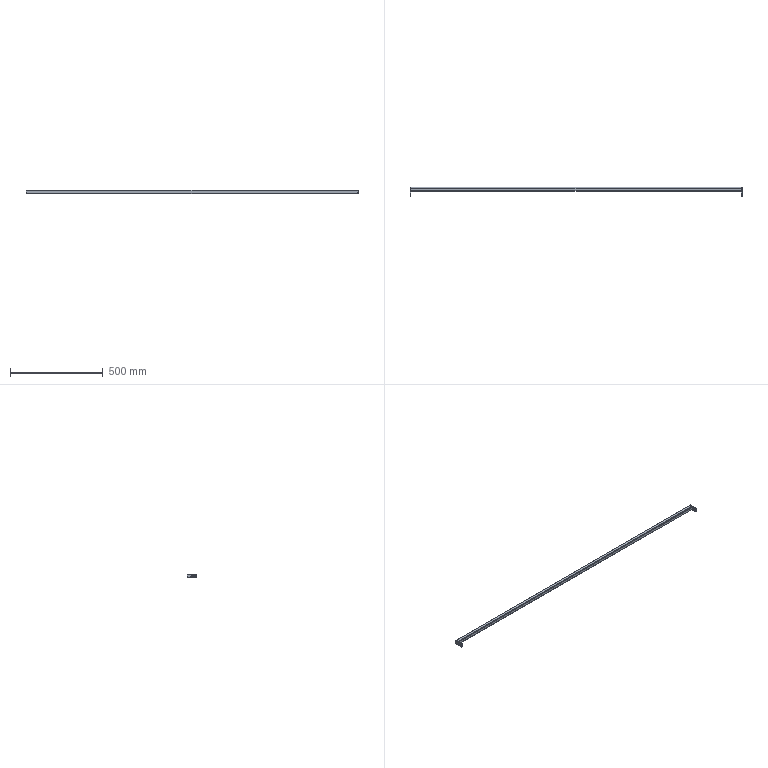Part | SolidWorks | features BaseBody 3 | 3 solids | 46 faces | box 1785 x 50 x 20 mm | volume 245964 mm3 | plane 30 | cylinder 16 | commonest cylinder face diameters 9 x8 4 x4 8 x4
STEP:
#1=CARTESIAN_POINT('',(1780.,-33.,-6.5));
#2=VERTEX_POINT('',#1);
#3=CARTESIAN_POINT('',(1780.,-33.,2.5));
#4=VERTEX_POINT('',#3);
#5=CARTESIAN_POINT('',(1780.,-33.,-2.));
#6=DIRECTION('',(-1.,0.,0.));
#7=DIRECTION('',(0.,0.,1.));
#8=AXIS2_PLACEMENT_3D('',#5,#6,#7);
#9=CIRCLE('',#8,4.5);
#10=EDGE_CURVE('',#2,#4,#9,.T.);
#11=ORIENTED_EDGE('',*,*,#10,.F.);
#12=CARTESIAN_POINT('',(1775.,-33.,-6.5));
#13=VERTEX_POINT('',#12);
#14=CARTESIAN_POINT('',(1775.,-33.,-6.5));
#15=DIRECTION('',(-1.,0.,0.));
#16=VECTOR('',#15,1000.);
#17=LINE('',#14,#16);
#18=EDGE_CURVE('',#2,#13,#17,.T.);
#19=ORIENTED_EDGE('',*,*,#18,.T.);
#20=CARTESIAN_POINT('',(1775.,-33.,2.5));
#21=VERTEX_POINT('',#20);
#22=CARTESIAN_POINT('',(1775.,-33.,-2.));
#23=DIRECTION('',(1.,0.,0.));
#24=DIRECTION('',(0.,0.,1.));
#25=AXIS2_PLACEMENT_3D('',#22,#23,#24);
#26=CIRCLE('',#25,4.5);
#27=EDGE_CURVE('',#21,#13,#26,.T.);
#28=ORIENTED_EDGE('',*,*,#27,.F.);
#29=CARTESIAN_POINT('',(1775.,-33.,2.5));
#30=DIRECTION('',(-1.,0.,0.));
#31=VECTOR('',#30,1000.);
#32=LINE('',#29,#31);
#33=EDGE_CURVE('',#4,#21,#32,.T.);
#34=ORIENTED_EDGE('',*,*,#33,.F.);
#35=EDGE_LOOP('',(#11,#19,#28,#34));
#36=FACE_OUTER_BOUND('',#35,.T.);
#37=CARTESIAN_POINT('',(1775.,-33.,-2.));
#38=DIRECTION('',(-1.,0.,0.));
#39=DIRECTION('',(0.,0.,1.));
#40=AXIS2_PLACEMENT_3D('',#37,#38,#39);
#41=CYLINDRICAL_SURFACE('',#40,4.5);
#42=ADVANCED_FACE('',(#36),#41,.F.);
#43=CARTESIAN_POINT('',(1780.,-18.,-6.5));
#44=VERTEX_POINT('',#43);
#45=CARTESIAN_POINT('',(1780.,-18.,2.5));
#46=VERTEX_POINT('',#45);
#47=CARTESIAN_POINT('',(1780.,-18.,-2.));
#48=DIRECTION('',(-1.,0.,0.));
#49=DIRECTION('',(0.,0.,1.));
#50=AXIS2_PLACEMENT_3D('',#47,#48,#49);
#51=CIRCLE('',#50,4.5);
#52=EDGE_CURVE('',#44,#46,#51,.T.);
#53=ORIENTED_EDGE('',*,*,#52,.F.);
#54=CARTESIAN_POINT('',(1775.,-18.,-6.5));
#55=VERTEX_POINT('',#54);
#56=CARTESIAN_POINT('',(1775.,-18.,-6.5));
#57=DIRECTION('',(-1.,0.,0.));
#58=VECTOR('',#57,1000.);
#59=LINE('',#56,#58);
#60=EDGE_CURVE('',#44,#55,#59,.T.);
#61=ORIENTED_EDGE('',*,*,#60,.T.);
#62=CARTESIAN_POINT('',(1775.,-18.,2.5));
#63=VERTEX_POINT('',#62);
#64=CARTESIAN_POINT('',(1775.,-18.,-2.));
#65=DIRECTION('',(1.,0.,0.));
#66=DIRECTION('',(0.,0.,1.));
#67=AXIS2_PLACEMENT_3D('',#64,#65,#66);
#68=CIRCLE('',#67,4.5);
#69=EDGE_CURVE('',#63,#55,#68,.T.);
#70=ORIENTED_EDGE('',*,*,#69,.F.);
#71=CARTESIAN_POINT('',(1775.,-18.,2.5));
#72=DIRECTION('',(-1.,0.,0.));
#73=VECTOR('',#72,1000.);
#74=LINE('',#71,#73);
#75=EDGE_CURVE('',#46,#63,#74,.T.);
#76=ORIENTED_EDGE('',*,*,#75,.F.);
#77=EDGE_LOOP('',(#53,#61,#70,#76));
#78=FACE_OUTER_BOUND('',#77,.T.);
#79=CARTESIAN_POINT('',(1775.,-18.,-2.));
#80=DIRECTION('',(-1.,0.,0.));
#81=DIRECTION('',(0.,0.,1.));
#82=AXIS2_PLACEMENT_3D('',#79,#80,#81);
#83=CYLINDRICAL_SURFACE('',#82,4.5);
#84=ADVANCED_FACE('',(#78),#83,.F.);
#85=CARTESIAN_POINT('',(1780.,10.,-8.));
#86=VERTEX_POINT('',#85);
#87=CARTESIAN_POINT('',(1780.,10.,8.));
#88=VERTEX_POINT('',#87);
#89=CARTESIAN_POINT('',(1780.,10.,0.));
#90=DIRECTION('',(0.,0.,1.));
#91=VECTOR('',#90,1000.);
#92=LINE('',#89,#91);
#93=EDGE_CURVE('',#86,#88,#92,.T.);
#94=ORIENTED_EDGE('',*,*,#93,.T.);
#95=CARTESIAN_POINT('',(1780.,8.,10.));
#96=VERTEX_POINT('',#95);
#97=CARTESIAN_POINT('',(1780.,10.,8.));
#98=DIRECTION('',(0.,-0.7071,0.7071));
#99=VECTOR('',#98,1000.);
#100=LINE('',#97,#99);
#101=EDGE_CURVE('',#88,#96,#100,.T.);
#102=ORIENTED_EDGE('',*,*,#101,.T.);
#103=CARTESIAN_POINT('',(1780.,-38.,10.));
#104=VERTEX_POINT('',#103);
#105=CARTESIAN_POINT('',(1780.,0.,10.));
#106=DIRECTION('',(0.,-1.,0.));
#107=VECTOR('',#106,1000.);
#108=LINE('',#105,#107);
#109=EDGE_CURVE('',#96,#104,#108,.T.);
#110=ORIENTED_EDGE('',*,*,#109,.T.);
#111=CARTESIAN_POINT('',(1780.,-40.,8.));
#112=VERTEX_POINT('',#111);
#113=CARTESIAN_POINT('',(1780.,-38.,10.));
#114=DIRECTION('',(0.,-0.7071,-0.7071));
#115=VECTOR('',#114,1000.);
#116=LINE('',#113,#115);
#117=EDGE_CURVE('',#104,#112,#116,.T.);
#118=ORIENTED_EDGE('',*,*,#117,.T.);
#119=CARTESIAN_POINT('',(1780.,-40.,-8.));
#120=VERTEX_POINT('',#119);
#121=CARTESIAN_POINT('',(1780.,-40.,0.));
#122=DIRECTION('',(0.,0.,-1.));
#123=VECTOR('',#122,1000.);
#124=LINE('',#121,#123);
#125=EDGE_CURVE('',#112,#120,#124,.T.);
#126=ORIENTED_EDGE('',*,*,#125,.T.);
#127=CARTESIAN_POINT('',(1780.,-38.,-10.));
#128=VERTEX_POINT('',#127);
#129=CARTESIAN_POINT('',(1780.,-40.,-8.));
#130=DIRECTION('',(0.,0.7071,-0.7071));
#131=VECTOR('',#130,1000.);
#132=LINE('',#129,#131);
#133=EDGE_CURVE('',#120,#128,#132,.T.);
#134=ORIENTED_EDGE('',*,*,#133,.T.);
#135=CARTESIAN_POINT('',(1780.,8.,-10.));
#136=VERTEX_POINT('',#135);
#137=CARTESIAN_POINT('',(1780.,0.,-10.));
#138=DIRECTION('',(0.,1.,0.));
#139=VECTOR('',#138,1000.);
#140=LINE('',#137,#139);
#141=EDGE_CURVE('',#128,#136,#140,.T.);
#142=ORIENTED_EDGE('',*,*,#141,.T.);
#143=CARTESIAN_POINT('',(1780.,8.,-10.));
#144=DIRECTION('',(0.,0.7071,0.7071));
#145=VECTOR('',#144,1000.);
#146=LINE('',#143,#145);
#147=EDGE_CURVE('',#136,#86,#146,.T.);
#148=ORIENTED_EDGE('',*,*,#147,.T.);
#149=EDGE_LOOP('',(#94,#102,#110,#118,#126,#134,#142,#148));
#150=FACE_OUTER_BOUND('',#149,.T.);
#151=CARTESIAN_POINT('',(1780.,-33.,-2.));
#152=DIRECTION('',(-1.,0.,0.));
#153=DIRECTION('',(0.,0.,1.));
#154=AXIS2_PLACEMENT_3D('',#151,#152,#153);
#155=CIRCLE('',#154,4.5);
#156=EDGE_CURVE('',#4,#2,#155,.T.);
#157=ORIENTED_EDGE('',*,*,#156,.T.);
#158=ORIENTED_EDGE('',*,*,#10,.T.);
#159=EDGE_LOOP('',(#157,#158));
#160=FACE_BOUND('',#159,.T.);
#161=CARTESIAN_POINT('',(1780.,-18.,-2.));
#162=DIRECTION('',(-1.,0.,0.));
#163=DIRECTION('',(0.,0.,1.));
#164=AXIS2_PLACEMENT_3D('',#161,#162,#163);
#165=CIRCLE('',#164,4.5);
#166=EDGE_CURVE('',#46,#44,#165,.T.);
#167=ORIENTED_EDGE('',*,*,#166,.T.);
#168=ORIENTED_EDGE('',*,*,#52,.T.);
#169=EDGE_LOOP('',(#167,#168));
#170=FACE_BOUND('',#169,.T.);
#171=CARTESIAN_POINT('',(1780.,0.,0.));
#172=DIRECTION('',(1.,0.,0.));
#173=DIRECTION('',(0.,0.,-1.));
#174=AXIS2_PLACEMENT_3D('',#171,#172,#173);
#175=PLANE('',#174);
#176=ADVANCED_FACE('',(#150,#160,#170),#175,.T.);
#177=CARTESIAN_POINT('',(1775.,10.,8.));
#178=VERTEX_POINT('',#177);
#179=CARTESIAN_POINT('',(1780.,10.,8.));
#180=DIRECTION('',(1.,0.,0.));
#181=VECTOR('',#180,1000.);
#182=LINE('',#179,#181);
#183=EDGE_CURVE('',#178,#88,#182,.T.);
#184=ORIENTED_EDGE('',*,*,#183,.F.);
#185=CARTESIAN_POINT('',(1775.,8.,10.));
#186=VERTEX_POINT('',#185);
#187=CARTESIAN_POINT('',(1775.,10.,8.));
#188=DIRECTION('',(0.,0.7071,-0.7071));
#189=VECTOR('',#188,1000.);
#190=LINE('',#187,#189);
#191=EDGE_CURVE('',#186,#178,#190,.T.);
#192=ORIENTED_EDGE('',*,*,#191,.F.);
#193=CARTESIAN_POINT('',(1780.,8.,10.));
#194=DIRECTION('',(-1.,0.,0.));
#195=VECTOR('',#194,1000.);
#196=LINE('',#193,#195);
#197=EDGE_CURVE('',#96,#186,#196,.T.);
#198=ORIENTED_EDGE('',*,*,#197,.F.);
#199=ORIENTED_EDGE('',*,*,#101,.F.);
#200=EDGE_LOOP('',(#184,#192,#198,#199));
#201=FACE_OUTER_BOUND('',#200,.T.);
#202=CARTESIAN_POINT('',(1780.,10.,8.));
#203=DIRECTION('',(0.,-0.7071,-0.7071));
#204=DIRECTION('',(0.,0.7071,-0.7071));
#205=AXIS2_PLACEMENT_3D('',#202,#203,#204);
#206=PLANE('',#205);
#207=ADVANCED_FACE('',(#201),#206,.F.);
#208=CARTESIAN_POINT('',(1775.,10.,-8.));
#209=VERTEX_POINT('',#208);
#210=CARTESIAN_POINT('',(1780.,10.,-8.));
#211=DIRECTION('',(1.,0.,0.));
#212=VECTOR('',#211,1000.);
#213=LINE('',#210,#212);
#214=EDGE_CURVE('',#209,#86,#213,.T.);
#215=ORIENTED_EDGE('',*,*,#214,.F.);
#216=CARTESIAN_POINT('',(1775.,10.,-10.));
#217=DIRECTION('',(0.,0.,-1.));
#218=VECTOR('',#217,1000.);
#219=LINE('',#216,#218);
#220=EDGE_CURVE('',#178,#209,#219,.T.);
#221=ORIENTED_EDGE('',*,*,#220,.F.);
#222=ORIENTED_EDGE('',*,*,#183,.T.);
#223=ORIENTED_EDGE('',*,*,#93,.F.);
#224=EDGE_LOOP('',(#215,#221,#222,#223));
#225=FACE_OUTER_BOUND('',#224,.T.);
#226=CARTESIAN_POINT('',(1780.,10.,-10.));
#227=DIRECTION('',(0.,-1.,0.));
#228=DIRECTION('',(0.,0.,-1.));
#229=AXIS2_PLACEMENT_3D('',#226,#227,#228);
#230=PLANE('',#229);
#231=ADVANCED_FACE('',(#225),#230,.F.);
#232=CARTESIAN_POINT('',(1775.,8.,-10.));
#233=VERTEX_POINT('',#232);
#234=CARTESIAN_POINT('',(1780.,8.,-10.));
#235=DIRECTION('',(1.,0.,0.));
#236=VECTOR('',#235,1000.);
#237=LINE('',#234,#236);
#238=EDGE_CURVE('',#233,#136,#237,.T.);
#239=ORIENTED_EDGE('',*,*,#238,.F.);
#240=CARTESIAN_POINT('',(1775.,8.,-10.));
#241=DIRECTION('',(0.,-0.7071,-0.7071));
#242=VECTOR('',#241,1000.);
#243=LINE('',#240,#242);
#244=EDGE_CURVE('',#209,#233,#243,.T.);
#245=ORIENTED_EDGE('',*,*,#244,.F.);
#246=ORIENTED_EDGE('',*,*,#214,.T.);
#247=ORIENTED_EDGE('',*,*,#147,.F.);
#248=EDGE_LOOP('',(#239,#245,#246,#247));
#249=FACE_OUTER_BOUND('',#248,.T.);
#250=CARTESIAN_POINT('',(1780.,8.,-10.));
#251=DIRECTION('',(0.,-0.7071,0.7071));
#252=DIRECTION('',(0.,-0.7071,-0.7071));
#253=AXIS2_PLACEMENT_3D('',#250,#251,#252);
#254=PLANE('',#253);
#255=ADVANCED_FACE('',(#249),#254,.F.);
#256=CARTESIAN_POINT('',(1775.,-38.,-10.));
#257=VERTEX_POINT('',#256);
#258=CARTESIAN_POINT('',(1780.,-38.,-10.));
#259=DIRECTION('',(1.,0.,0.));
#260=VECTOR('',#259,1000.);
#261=LINE('',#258,#260);
#262=EDGE_CURVE('',#257,#128,#261,.T.);
#263=ORIENTED_EDGE('',*,*,#262,.F.);
#264=CARTESIAN_POINT('',(1775.,10.,-10.));
#265=DIRECTION('',(0.,-1.,0.));
#266=VECTOR('',#265,1000.);
#267=LINE('',#264,#266);
#268=EDGE_CURVE('',#233,#257,#267,.T.);
#269=ORIENTED_EDGE('',*,*,#268,.F.);
#270=ORIENTED_EDGE('',*,*,#238,.T.);
#271=ORIENTED_EDGE('',*,*,#141,.F.);
#272=EDGE_LOOP('',(#263,#269,#270,#271));
#273=FACE_OUTER_BOUND('',#272,.T.);
#274=CARTESIAN_POINT('',(1780.,10.,-10.));
#275=DIRECTION('',(0.,0.,1.));
#276=DIRECTION('',(0.,-1.,0.));
#277=AXIS2_PLACEMENT_3D('',#274,#275,#276);
#278=PLANE('',#277);
#279=ADVANCED_FACE('',(#273),#278,.F.);
#280=CARTESIAN_POINT('',(1775.,-40.,-8.));
#281=VERTEX_POINT('',#280);
#282=CARTESIAN_POINT('',(1780.,-40.,-8.));
#283=DIRECTION('',(1.,0.,0.));
#284=VECTOR('',#283,1000.);
#285=LINE('',#282,#284);
#286=EDGE_CURVE('',#281,#120,#285,.T.);
#287=ORIENTED_EDGE('',*,*,#286,.F.);
#288=CARTESIAN_POINT('',(1775.,-40.,-8.));
#289=DIRECTION('',(0.,-0.7071,0.7071));
#290=VECTOR('',#289,1000.);
#291=LINE('',#288,#290);
#292=EDGE_CURVE('',#257,#281,#291,.T.);
#293=ORIENTED_EDGE('',*,*,#292,.F.);
#294=ORIENTED_EDGE('',*,*,#262,.T.);
#295=ORIENTED_EDGE('',*,*,#133,.F.);
#296=EDGE_LOOP('',(#287,#293,#294,#295));
#297=FACE_OUTER_BOUND('',#296,.T.);
#298=CARTESIAN_POINT('',(1780.,-40.,-8.));
#299=DIRECTION('',(0.,0.7071,0.7071));
#300=DIRECTION('',(0.,-0.7071,0.7071));
#301=AXIS2_PLACEMENT_3D('',#298,#299,#300);
#302=PLANE('',#301);
#303=ADVANCED_FACE('',(#297),#302,.F.);
#304=CARTESIAN_POINT('',(1775.,-40.,8.));
#305=VERTEX_POINT('',#304);
#306=CARTESIAN_POINT('',(1780.,-40.,8.));
#307=DIRECTION('',(1.,0.,0.));
#308=VECTOR('',#307,1000.);
#309=LINE('',#306,#308);
#310=EDGE_CURVE('',#305,#112,#309,.T.);
#311=ORIENTED_EDGE('',*,*,#310,.F.);
#312=CARTESIAN_POINT('',(1775.,-40.,-10.));
#313=DIRECTION('',(0.,0.,1.));
#314=VECTOR('',#313,1000.);
#315=LINE('',#312,#314);
#316=EDGE_CURVE('',#281,#305,#315,.T.);
#317=ORIENTED_EDGE('',*,*,#316,.F.);
#318=ORIENTED_EDGE('',*,*,#286,.T.);
#319=ORIENTED_EDGE('',*,*,#125,.F.);
#320=EDGE_LOOP('',(#311,#317,#318,#319));
#321=FACE_OUTER_BOUND('',#320,.T.);
#322=CARTESIAN_POINT('',(1780.,-40.,-10.));
#323=DIRECTION('',(0.,1.,0.));
#324=DIRECTION('',(0.,0.,1.));
#325=AXIS2_PLACEMENT_3D('',#322,#323,#324);
#326=PLANE('',#325);
#327=ADVANCED_FACE('',(#321),#326,.F.);
#328=CARTESIAN_POINT('',(1775.,-38.,10.));
#329=VERTEX_POINT('',#328);
#330=CARTESIAN_POINT('',(1780.,-38.,10.));
#331=DIRECTION('',(1.,0.,0.));
#332=VECTOR('',#331,1000.);
#333=LINE('',#330,#332);
#334=EDGE_CURVE('',#329,#104,#333,.T.);
#335=ORIENTED_EDGE('',*,*,#334,.F.);
#336=CARTESIAN_POINT('',(1775.,-38.,10.));
#337=DIRECTION('',(0.,0.7071,0.7071));
#338=VECTOR('',#337,1000.);
#339=LINE('',#336,#338);
#340=EDGE_CURVE('',#305,#329,#339,.T.);
#341=ORIENTED_EDGE('',*,*,#340,.F.);
#342=ORIENTED_EDGE('',*,*,#310,.T.);
#343=ORIENTED_EDGE('',*,*,#117,.F.);
#344=EDGE_LOOP('',(#335,#341,#342,#343));
#345=FACE_OUTER_BOUND('',#344,.T.);
#346=CARTESIAN_POINT('',(1780.,-38.,10.));
#347=DIRECTION('',(0.,0.7071,-0.7071));
#348=DIRECTION('',(0.,0.7071,0.7071));
#349=AXIS2_PLACEMENT_3D('',#346,#347,#348);
#350=PLANE('',#349);
#351=ADVANCED_FACE('',(#345),#350,.F.);
#352=ORIENTED_EDGE('',*,*,#334,.T.);
#353=ORIENTED_EDGE('',*,*,#109,.F.);
#354=ORIENTED_EDGE('',*,*,#197,.T.);
#355=CARTESIAN_POINT('',(1775.,10.,10.));
#356=DIRECTION('',(0.,1.,0.));
#357=VECTOR('',#356,1000.);
#358=LINE('',#355,#357);
#359=EDGE_CURVE('',#329,#186,#358,.T.);
#360=ORIENTED_EDGE('',*,*,#359,.F.);
#361=EDGE_LOOP('',(#352,#353,#354,#360));
#362=FACE_OUTER_BOUND('',#361,.T.);
#363=CARTESIAN_POINT('',(1780.,10.,10.));
#364=DIRECTION('',(0.,0.,-1.));
#365=DIRECTION('',(0.,1.,0.));
#366=AXIS2_PLACEMENT_3D('',#363,#364,#365);
#367=PLANE('',#366);
#368=ADVANCED_FACE('',(#362),#367,.F.);
#369=ORIENTED_EDGE('',*,*,#18,.F.);
#370=ORIENTED_EDGE('',*,*,#156,.F.);
#371=ORIENTED_EDGE('',*,*,#33,.T.);
#372=CARTESIAN_POINT('',(1775.,-33.,-2.));
#373=DIRECTION('',(1.,0.,0.));
#374=DIRECTION('',(0.,0.,1.));
#375=AXIS2_PLACEMENT_3D('',#372,#373,#374);
#376=CIRCLE('',#375,4.5);
#377=EDGE_CURVE('',#13,#21,#376,.T.);
#378=ORIENTED_EDGE('',*,*,#377,.F.);
#379=EDGE_LOOP('',(#369,#370,#371,#378));
#380=FACE_OUTER_BOUND('',#379,.T.);
#381=CARTESIAN_POINT('',(1775.,-33.,-2.));
#382=DIRECTION('',(-1.,0.,0.));
#383=DIRECTION('',(0.,0.,1.));
#384=AXIS2_PLACEMENT_3D('',#381,#382,#383);
#385=CYLINDRICAL_SURFACE('',#384,4.5);
#386=ADVANCED_FACE('',(#380),#385,.F.);
#387=ORIENTED_EDGE('',*,*,#60,.F.);
#388=ORIENTED_EDGE('',*,*,#166,.F.);
#389=ORIENTED_EDGE('',*,*,#75,.T.);
#390=CARTESIAN_POINT('',(1775.,-18.,-2.));
#391=DIRECTION('',(1.,0.,0.));
#392=DIRECTION('',(0.,0.,1.));
#393=AXIS2_PLACEMENT_3D('',#390,#391,#392);
#394=CIRCLE('',#393,4.5);
#395=EDGE_CURVE('',#55,#63,#394,.T.);
#396=ORIENTED_EDGE('',*,*,#395,.F.);
#397=EDGE_LOOP('',(#387,#388,#389,#396));
#398=FACE_OUTER_BOUND('',#397,.T.);
#399=CARTESIAN_POINT('',(1775.,-18.,-2.));
#400=DIRECTION('',(-1.,0.,0.));
#401=DIRECTION('',(0.,0.,1.));
#402=AXIS2_PLACEMENT_3D('',#399,#400,#401);
#403=CYLINDRICAL_SURFACE('',#402,4.5);
#404=ADVANCED_FACE('',(#398),#403,.F.);
#405=ORIENTED_EDGE('',*,*,#244,.T.);
#406=ORIENTED_EDGE('',*,*,#268,.T.);
#407=ORIENTED_EDGE('',*,*,#292,.T.);
#408=ORIENTED_EDGE('',*,*,#316,.T.);
#409=ORIENTED_EDGE('',*,*,#340,.T.);
#410=ORIENTED_EDGE('',*,*,#359,.T.);
#411=ORIENTED_EDGE('',*,*,#191,.T.);
#412=ORIENTED_EDGE('',*,*,#220,.T.);
#413=EDGE_LOOP('',(#405,#406,#407,#408,#409,#410,#411,#412));
#414=FACE_OUTER_BOUND('',#413,.T.);
#415=ORIENTED_EDGE('',*,*,#27,.T.);
#416=ORIENTED_EDGE('',*,*,#377,.T.);
#417=EDGE_LOOP('',(#415,#416));
#418=FACE_BOUND('',#417,.T.);
#419=ORIENTED_EDGE('',*,*,#69,.T.);
#420=ORIENTED_EDGE('',*,*,#395,.T.);
#421=EDGE_LOOP('',(#419,#420));
#422=FACE_BOUND('',#421,.T.);
#423=CARTESIAN_POINT('',(1775.,0.,0.));
#424=DIRECTION('',(1.,0.,0.));
#425=DIRECTION('',(0.,0.,-1.));
#426=AXIS2_PLACEMENT_3D('',#423,#424,#425);
#427=PLANE('',#426);
#428=ADVANCED_FACE('',(#414,#418,#422),#427,.F.);
#429=CLOSED_SHELL('',(#42,#84,#176,#207,#231,#255,#279,#303,#327,#351,#368,#386,#404,#428));
#430=MANIFOLD_SOLID_BREP('',#429);
#431=CARTESIAN_POINT('',(-5.,-33.,2.5));
#432=VERTEX_POINT('',#431);
#433=CARTESIAN_POINT('',(-5.,-33.,-6.5));
#434=VERTEX_POINT('',#433);
#435=CARTESIAN_POINT('',(-5.,-33.,-2.));
#436=DIRECTION('',(1.,0.,0.));
#437=DIRECTION('',(0.,0.,-1.));
#438=AXIS2_PLACEMENT_3D('',#435,#436,#437);
#439=CIRCLE('',#438,4.5);
#440=EDGE_CURVE('',#432,#434,#439,.T.);
#441=ORIENTED_EDGE('',*,*,#440,.F.);
#442=CARTESIAN_POINT('',(0.,-33.,2.5));
#443=VERTEX_POINT('',#442);
#444=CARTESIAN_POINT('',(0.,-33.,2.5));
#445=DIRECTION('',(1.,0.,0.));
#446=VECTOR('',#445,1000.);
#447=LINE('',#444,#446);
#448=EDGE_CURVE('',#432,#443,#447,.T.);
#449=ORIENTED_EDGE('',*,*,#448,.T.);
#450=CARTESIAN_POINT('',(0.,-33.,-6.5));
#451=VERTEX_POINT('',#450);
#452=CARTESIAN_POINT('',(0.,-33.,-2.));
#453=DIRECTION('',(1.,0.,0.));
#454=DIRECTION('',(0.,0.,-1.));
#455=AXIS2_PLACEMENT_3D('',#452,#453,#454);
#456=CIRCLE('',#455,4.5);
#457=EDGE_CURVE('',#443,#451,#456,.T.);
#458=ORIENTED_EDGE('',*,*,#457,.T.);
#459=CARTESIAN_POINT('',(0.,-33.,-6.5));
#460=DIRECTION('',(1.,0.,0.));
#461=VECTOR('',#460,1000.);
#462=LINE('',#459,#461);
#463=EDGE_CURVE('',#434,#451,#462,.T.);
#464=ORIENTED_EDGE('',*,*,#463,.F.);
#465=EDGE_LOOP('',(#441,#449,#458,#464));
#466=FACE_OUTER_BOUND('',#465,.T.);
#467=CARTESIAN_POINT('',(0.,-33.,-2.));
#468=DIRECTION('',(1.,0.,0.));
#469=DIRECTION('',(0.,0.,-1.));
#470=AXIS2_PLACEMENT_3D('',#467,#468,#469);
#471=CYLINDRICAL_SURFACE('',#470,4.5);
#472=ADVANCED_FACE('',(#466),#471,.F.);
#473=CARTESIAN_POINT('',(-5.,-18.,2.5));
#474=VERTEX_POINT('',#473);
#475=CARTESIAN_POINT('',(-5.,-18.,-6.5));
#476=VERTEX_POINT('',#475);
#477=CARTESIAN_POINT('',(-5.,-18.,-2.));
#478=DIRECTION('',(1.,0.,0.));
#479=DIRECTION('',(0.,0.,-1.));
#480=AXIS2_PLACEMENT_3D('',#477,#478,#479);
#481=CIRCLE('',#480,4.5);
#482=EDGE_CURVE('',#474,#476,#481,.T.);
#483=ORIENTED_EDGE('',*,*,#482,.F.);
#484=CARTESIAN_POINT('',(0.,-18.,2.5));
#485=VERTEX_POINT('',#484);
#486=CARTESIAN_POINT('',(0.,-18.,2.5));
#487=DIRECTION('',(1.,0.,0.));
#488=VECTOR('',#487,1000.);
#489=LINE('',#486,#488);
#490=EDGE_CURVE('',#474,#485,#489,.T.);
#491=ORIENTED_EDGE('',*,*,#490,.T.);
#492=CARTESIAN_POINT('',(0.,-18.,-6.5));
#493=VERTEX_POINT('',#492);
#494=CARTESIAN_POINT('',(0.,-18.,-2.));
#495=DIRECTION('',(1.,0.,0.));
#496=DIRECTION('',(0.,0.,-1.));
#497=AXIS2_PLACEMENT_3D('',#494,#495,#496);
#498=CIRCLE('',#497,4.5);
#499=EDGE_CURVE('',#485,#493,#498,.T.);
#500=ORIENTED_EDGE('',*,*,#499,.T.);
#501=CARTESIAN_POINT('',(0.,-18.,-6.5));
#502=DIRECTION('',(1.,0.,0.));
#503=VECTOR('',#502,1000.);
#504=LINE('',#501,#503);
#505=EDGE_CURVE('',#476,#493,#504,.T.);
#506=ORIENTED_EDGE('',*,*,#505,.F.);
#507=EDGE_LOOP('',(#483,#491,#500,#506));
#508=FACE_OUTER_BOUND('',#507,.T.);
#509=CARTESIAN_POINT('',(0.,-18.,-2.));
#510=DIRECTION('',(1.,0.,0.));
#511=DIRECTION('',(0.,0.,-1.));
#512=AXIS2_PLACEMENT_3D('',#509,#510,#511);
#513=CYLINDRICAL_SURFACE('',#512,4.5);
#514=ADVANCED_FACE('',(#508),#513,.F.);
#515=CARTESIAN_POINT('',(0.,8.,10.));
#516=VERTEX_POINT('',#515);
#517=CARTESIAN_POINT('',(0.,10.,8.));
#518=VERTEX_POINT('',#517);
#519=CARTESIAN_POINT('',(0.,8.,10.));
#520=DIRECTION('',(0.,0.7071,-0.7071));
#521=VECTOR('',#520,1000.);
#522=LINE('',#519,#521);
#523=EDGE_CURVE('',#516,#518,#522,.T.);
#524=ORIENTED_EDGE('',*,*,#523,.F.);
#525=CARTESIAN_POINT('',(0.,-38.,10.));
#526=VERTEX_POINT('',#525);
#527=CARTESIAN_POINT('',(0.,0.,10.));
#528=DIRECTION('',(0.,1.,0.));
#529=VECTOR('',#528,1000.);
#530=LINE('',#527,#529);
#531=EDGE_CURVE('',#526,#516,#530,.T.);
#532=ORIENTED_EDGE('',*,*,#531,.F.);
#533=CARTESIAN_POINT('',(0.,-40.,8.));
#534=VERTEX_POINT('',#533);
#535=CARTESIAN_POINT('',(0.,-40.,8.));
#536=DIRECTION('',(0.,0.7071,0.7071));
#537=VECTOR('',#536,1000.);
#538=LINE('',#535,#537);
#539=EDGE_CURVE('',#534,#526,#538,.T.);
#540=ORIENTED_EDGE('',*,*,#539,.F.);
#541=CARTESIAN_POINT('',(0.,-40.,-8.));
#542=VERTEX_POINT('',#541);
#543=CARTESIAN_POINT('',(0.,-40.,0.));
#544=DIRECTION('',(0.,0.,1.));
#545=VECTOR('',#544,1000.);
#546=LINE('',#543,#545);
#547=EDGE_CURVE('',#542,#534,#546,.T.);
#548=ORIENTED_EDGE('',*,*,#547,.F.);
#549=CARTESIAN_POINT('',(0.,-38.,-10.));
#550=VERTEX_POINT('',#549);
#551=CARTESIAN_POINT('',(0.,-38.,-10.));
#552=DIRECTION('',(0.,-0.7071,0.7071));
#553=VECTOR('',#552,1000.);
#554=LINE('',#551,#553);
#555=EDGE_CURVE('',#550,#542,#554,.T.);
#556=ORIENTED_EDGE('',*,*,#555,.F.);
#557=CARTESIAN_POINT('',(0.,8.,-10.));
#558=VERTEX_POINT('',#557);
#559=CARTESIAN_POINT('',(0.,0.,-10.));
#560=DIRECTION('',(0.,-1.,0.));
#561=VECTOR('',#560,1000.);
#562=LINE('',#559,#561);
#563=EDGE_CURVE('',#558,#550,#562,.T.);
#564=ORIENTED_EDGE('',*,*,#563,.F.);
#565=CARTESIAN_POINT('',(0.,10.,-8.));
#566=VERTEX_POINT('',#565);
#567=CARTESIAN_POINT('',(0.,10.,-8.));
#568=DIRECTION('',(0.,-0.7071,-0.7071));
#569=VECTOR('',#568,1000.);
#570=LINE('',#567,#569);
#571=EDGE_CURVE('',#566,#558,#570,.T.);
#572=ORIENTED_EDGE('',*,*,#571,.F.);
#573=CARTESIAN_POINT('',(0.,10.,0.));
#574=DIRECTION('',(0.,0.,-1.));
#575=VECTOR('',#574,1000.);
#576=LINE('',#573,#575);
#577=EDGE_CURVE('',#518,#566,#576,.T.);
#578=ORIENTED_EDGE('',*,*,#577,.F.);
#579=EDGE_LOOP('',(#524,#532,#540,#548,#556,#564,#572,#578));
#580=FACE_OUTER_BOUND('',#579,.T.);
#581=CARTESIAN_POINT('',(0.,-33.,-2.));
#582=DIRECTION('',(1.,0.,0.));
#583=DIRECTION('',(0.,0.,-1.));
#584=AXIS2_PLACEMENT_3D('',#581,#582,#583);
#585=CIRCLE('',#584,4.5);
#586=EDGE_CURVE('',#451,#443,#585,.T.);
#587=ORIENTED_EDGE('',*,*,#586,.F.);
#588=ORIENTED_EDGE('',*,*,#457,.F.);
#589=EDGE_LOOP('',(#587,#588));
#590=FACE_BOUND('',#589,.T.);
#591=CARTESIAN_POINT('',(0.,-18.,-2.));
#592=DIRECTION('',(1.,0.,0.));
#593=DIRECTION('',(0.,0.,-1.));
#594=AXIS2_PLACEMENT_3D('',#591,#592,#593);
#595=CIRCLE('',#594,4.5);
#596=EDGE_CURVE('',#493,#485,#595,.T.);
#597=ORIENTED_EDGE('',*,*,#596,.F.);
#598=ORIENTED_EDGE('',*,*,#499,.F.);
#599=EDGE_LOOP('',(#597,#598));
#600=FACE_BOUND('',#599,.T.);
#601=CARTESIAN_POINT('',(0.,0.,0.));
#602=DIRECTION('',(-1.,0.,0.));
#603=DIRECTION('',(0.,0.,1.));
#604=AXIS2_PLACEMENT_3D('',#601,#602,#603);
#605=PLANE('',#604);
#606=ADVANCED_FACE('',(#580,#590,#600),#605,.F.);
#607=CARTESIAN_POINT('',(-5.,10.,8.));
#608=VERTEX_POINT('',#607);
#609=CARTESIAN_POINT('',(-5.,10.,8.));
#610=DIRECTION('',(-1.,0.,0.));
#611=VECTOR('',#610,1000.);
#612=LINE('',#609,#611);
#613=EDGE_CURVE('',#518,#608,#612,.T.);
#614=ORIENTED_EDGE('',*,*,#613,.F.);
#615=ORIENTED_EDGE('',*,*,#577,.T.);
#616=CARTESIAN_POINT('',(-5.,10.,-8.));
#617=VERTEX_POINT('',#616);
#618=CARTESIAN_POINT('',(-5.,10.,-8.));
#619=DIRECTION('',(1.,0.,0.));
#620=VECTOR('',#619,1000.);
#621=LINE('',#618,#620);
#622=EDGE_CURVE('',#617,#566,#621,.T.);
#623=ORIENTED_EDGE('',*,*,#622,.F.);
#624=CARTESIAN_POINT('',(-5.,10.,-10.));
#625=DIRECTION('',(0.,0.,-1.));
#626=VECTOR('',#625,1000.);
#627=LINE('',#624,#626);
#628=EDGE_CURVE('',#608,#617,#627,.T.);
#629=ORIENTED_EDGE('',*,*,#628,.F.);
#630=EDGE_LOOP('',(#614,#615,#623,#629));
#631=FACE_OUTER_BOUND('',#630,.T.);
#632=CARTESIAN_POINT('',(-5.,10.,-10.));
#633=DIRECTION('',(0.,-1.,0.));
#634=DIRECTION('',(0.,0.,-1.));
#635=AXIS2_PLACEMENT_3D('',#632,#633,#634);
#636=PLANE('',#635);
#637=ADVANCED_FACE('',(#631),#636,.F.);
#638=CARTESIAN_POINT('',(-5.,8.,10.));
#639=VERTEX_POINT('',#638);
#640=CARTESIAN_POINT('',(-5.,8.,10.));
#641=DIRECTION('',(-1.,0.,0.));
#642=VECTOR('',#641,1000.);
#643=LINE('',#640,#642);
#644=EDGE_CURVE('',#516,#639,#643,.T.);
#645=ORIENTED_EDGE('',*,*,#644,.F.);
#646=ORIENTED_EDGE('',*,*,#523,.T.);
#647=ORIENTED_EDGE('',*,*,#613,.T.);
#648=CARTESIAN_POINT('',(-5.,10.,8.));
#649=DIRECTION('',(0.,0.7071,-0.7071));
#650=VECTOR('',#649,1000.);
#651=LINE('',#648,#650);
#652=EDGE_CURVE('',#639,#608,#651,.T.);
#653=ORIENTED_EDGE('',*,*,#652,.F.);
#654=EDGE_LOOP('',(#645,#646,#647,#653));
#655=FACE_OUTER_BOUND('',#654,.T.);
#656=CARTESIAN_POINT('',(-5.,10.,8.));
#657=DIRECTION('',(0.,-0.7071,-0.7071));
#658=DIRECTION('',(0.,0.7071,-0.7071));
#659=AXIS2_PLACEMENT_3D('',#656,#657,#658);
#660=PLANE('',#659);
#661=ADVANCED_FACE('',(#655),#660,.F.);
#662=ORIENTED_EDGE('',*,*,#644,.T.);
#663=CARTESIAN_POINT('',(-5.,-38.,10.));
#664=VERTEX_POINT('',#663);
#665=CARTESIAN_POINT('',(-5.,10.,10.));
#666=DIRECTION('',(0.,1.,0.));
#667=VECTOR('',#666,1000.);
#668=LINE('',#665,#667);
#669=EDGE_CURVE('',#664,#639,#668,.T.);
#670=ORIENTED_EDGE('',*,*,#669,.F.);
#671=CARTESIAN_POINT('',(-5.,-38.,10.));
#672=DIRECTION('',(-1.,0.,0.));
#673=VECTOR('',#672,1000.);
#674=LINE('',#671,#673);
#675=EDGE_CURVE('',#526,#664,#674,.T.);
#676=ORIENTED_EDGE('',*,*,#675,.F.);
#677=ORIENTED_EDGE('',*,*,#531,.T.);
#678=EDGE_LOOP('',(#662,#670,#676,#677));
#679=FACE_OUTER_BOUND('',#678,.T.);
#680=CARTESIAN_POINT('',(-5.,10.,10.));
#681=DIRECTION('',(0.,0.,-1.));
#682=DIRECTION('',(0.,1.,0.));
#683=AXIS2_PLACEMENT_3D('',#680,#681,#682);
#684=PLANE('',#683);
#685=ADVANCED_FACE('',(#679),#684,.F.);
#686=CARTESIAN_POINT('',(-5.,-40.,8.));
#687=VERTEX_POINT('',#686);
#688=CARTESIAN_POINT('',(-5.,-40.,8.));
#689=DIRECTION('',(-1.,0.,0.));
#690=VECTOR('',#689,1000.);
#691=LINE('',#688,#690);
#692=EDGE_CURVE('',#534,#687,#691,.T.);
#693=ORIENTED_EDGE('',*,*,#692,.F.);
#694=ORIENTED_EDGE('',*,*,#539,.T.);
#695=ORIENTED_EDGE('',*,*,#675,.T.);
#696=CARTESIAN_POINT('',(-5.,-38.,10.));
#697=DIRECTION('',(0.,0.7071,0.7071));
#698=VECTOR('',#697,1000.);
#699=LINE('',#696,#698);
#700=EDGE_CURVE('',#687,#664,#699,.T.);
#701=ORIENTED_EDGE('',*,*,#700,.F.);
#702=EDGE_LOOP('',(#693,#694,#695,#701));
#703=FACE_OUTER_BOUND('',#702,.T.);
#704=CARTESIAN_POINT('',(-5.,-38.,10.));
#705=DIRECTION('',(0.,0.7071,-0.7071));
#706=DIRECTION('',(0.,0.7071,0.7071));
#707=AXIS2_PLACEMENT_3D('',#704,#705,#706);
#708=PLANE('',#707);
#709=ADVANCED_FACE('',(#703),#708,.F.);
#710=CARTESIAN_POINT('',(-5.,-40.,-8.));
#711=VERTEX_POINT('',#710);
#712=CARTESIAN_POINT('',(-5.,-40.,-8.));
#713=DIRECTION('',(-1.,0.,0.));
#714=VECTOR('',#713,1000.);
#715=LINE('',#712,#714);
#716=EDGE_CURVE('',#542,#711,#715,.T.);
#717=ORIENTED_EDGE('',*,*,#716,.F.);
#718=ORIENTED_EDGE('',*,*,#547,.T.);
#719=ORIENTED_EDGE('',*,*,#692,.T.);
#720=CARTESIAN_POINT('',(-5.,-40.,-10.));
#721=DIRECTION('',(0.,0.,1.));
#722=VECTOR('',#721,1000.);
#723=LINE('',#720,#722);
#724=EDGE_CURVE('',#711,#687,#723,.T.);
#725=ORIENTED_EDGE('',*,*,#724,.F.);
#726=EDGE_LOOP('',(#717,#718,#719,#725));
#727=FACE_OUTER_BOUND('',#726,.T.);
#728=CARTESIAN_POINT('',(-5.,-40.,-10.));
#729=DIRECTION('',(0.,1.,0.));
#730=DIRECTION('',(0.,0.,1.));
#731=AXIS2_PLACEMENT_3D('',#728,#729,#730);
#732=PLANE('',#731);
#733=ADVANCED_FACE('',(#727),#732,.F.);
#734=CARTESIAN_POINT('',(-5.,-38.,-10.));
#735=VERTEX_POINT('',#734);
#736=CARTESIAN_POINT('',(-5.,-38.,-10.));
#737=DIRECTION('',(-1.,0.,0.));
#738=VECTOR('',#737,1000.);
#739=LINE('',#736,#738);
#740=EDGE_CURVE('',#550,#735,#739,.T.);
#741=ORIENTED_EDGE('',*,*,#740,.F.);
#742=ORIENTED_EDGE('',*,*,#555,.T.);
#743=ORIENTED_EDGE('',*,*,#716,.T.);
#744=CARTESIAN_POINT('',(-5.,-40.,-8.));
#745=DIRECTION('',(0.,-0.7071,0.7071));
#746=VECTOR('',#745,1000.);
#747=LINE('',#744,#746);
#748=EDGE_CURVE('',#735,#711,#747,.T.);
#749=ORIENTED_EDGE('',*,*,#748,.F.);
#750=EDGE_LOOP('',(#741,#742,#743,#749));
#751=FACE_OUTER_BOUND('',#750,.T.);
#752=CARTESIAN_POINT('',(-5.,-40.,-8.));
#753=DIRECTION('',(0.,0.7071,0.7071));
#754=DIRECTION('',(0.,-0.7071,0.7071));
#755=AXIS2_PLACEMENT_3D('',#752,#753,#754);
#756=PLANE('',#755);
#757=ADVANCED_FACE('',(#751),#756,.F.);
#758=CARTESIAN_POINT('',(-5.,8.,-10.));
#759=VERTEX_POINT('',#758);
#760=CARTESIAN_POINT('',(-5.,8.,-10.));
#761=DIRECTION('',(-1.,0.,0.));
#762=VECTOR('',#761,1000.);
#763=LINE('',#760,#762);
#764=EDGE_CURVE('',#558,#759,#763,.T.);
#765=ORIENTED_EDGE('',*,*,#764,.F.);
#766=ORIENTED_EDGE('',*,*,#563,.T.);
#767=ORIENTED_EDGE('',*,*,#740,.T.);
#768=CARTESIAN_POINT('',(-5.,10.,-10.));
#769=DIRECTION('',(0.,-1.,0.));
#770=VECTOR('',#769,1000.);
#771=LINE('',#768,#770);
#772=EDGE_CURVE('',#759,#735,#771,.T.);
#773=ORIENTED_EDGE('',*,*,#772,.F.);
#774=EDGE_LOOP('',(#765,#766,#767,#773));
#775=FACE_OUTER_BOUND('',#774,.T.);
#776=CARTESIAN_POINT('',(-5.,10.,-10.));
#777=DIRECTION('',(0.,0.,1.));
#778=DIRECTION('',(0.,-1.,0.));
#779=AXIS2_PLACEMENT_3D('',#776,#777,#778);
#780=PLANE('',#779);
#781=ADVANCED_FACE('',(#775),#780,.F.);
#782=ORIENTED_EDGE('',*,*,#622,.T.);
#783=ORIENTED_EDGE('',*,*,#571,.T.);
#784=ORIENTED_EDGE('',*,*,#764,.T.);
#785=CARTESIAN_POINT('',(-5.,8.,-10.));
#786=DIRECTION('',(0.,-0.7071,-0.7071));
#787=VECTOR('',#786,1000.);
#788=LINE('',#785,#787);
#789=EDGE_CURVE('',#617,#759,#788,.T.);
#790=ORIENTED_EDGE('',*,*,#789,.F.);
#791=EDGE_LOOP('',(#782,#783,#784,#790));
#792=FACE_OUTER_BOUND('',#791,.T.);
#793=CARTESIAN_POINT('',(-5.,8.,-10.));
#794=DIRECTION('',(0.,-0.7071,0.7071));
#795=DIRECTION('',(0.,-0.7071,-0.7071));
#796=AXIS2_PLACEMENT_3D('',#793,#794,#795);
#797=PLANE('',#796);
#798=ADVANCED_FACE('',(#792),#797,.F.);
#799=ORIENTED_EDGE('',*,*,#448,.F.);
#800=CARTESIAN_POINT('',(-5.,-33.,-2.));
#801=DIRECTION('',(1.,0.,0.));
#802=DIRECTION('',(0.,0.,-1.));
#803=AXIS2_PLACEMENT_3D('',#800,#801,#802);
#804=CIRCLE('',#803,4.5);
#805=EDGE_CURVE('',#434,#432,#804,.T.);
#806=ORIENTED_EDGE('',*,*,#805,.F.);
#807=ORIENTED_EDGE('',*,*,#463,.T.);
#808=ORIENTED_EDGE('',*,*,#586,.T.);
#809=EDGE_LOOP('',(#799,#806,#807,#808));
#810=FACE_OUTER_BOUND('',#809,.T.);
#811=CARTESIAN_POINT('',(0.,-33.,-2.));
#812=DIRECTION('',(1.,0.,0.));
#813=DIRECTION('',(0.,0.,-1.));
#814=AXIS2_PLACEMENT_3D('',#811,#812,#813);
#815=CYLINDRICAL_SURFACE('',#814,4.5);
#816=ADVANCED_FACE('',(#810),#815,.F.);
#817=ORIENTED_EDGE('',*,*,#490,.F.);
#818=CARTESIAN_POINT('',(-5.,-18.,-2.));
#819=DIRECTION('',(1.,0.,0.));
#820=DIRECTION('',(0.,0.,-1.));
#821=AXIS2_PLACEMENT_3D('',#818,#819,#820);
#822=CIRCLE('',#821,4.5);
#823=EDGE_CURVE('',#476,#474,#822,.T.);
#824=ORIENTED_EDGE('',*,*,#823,.F.);
#825=ORIENTED_EDGE('',*,*,#505,.T.);
#826=ORIENTED_EDGE('',*,*,#596,.T.);
#827=EDGE_LOOP('',(#817,#824,#825,#826));
#828=FACE_OUTER_BOUND('',#827,.T.);
#829=CARTESIAN_POINT('',(0.,-18.,-2.));
#830=DIRECTION('',(1.,0.,0.));
#831=DIRECTION('',(0.,0.,-1.));
#832=AXIS2_PLACEMENT_3D('',#829,#830,#831);
#833=CYLINDRICAL_SURFACE('',#832,4.5);
#834=ADVANCED_FACE('',(#828),#833,.F.);
#835=ORIENTED_EDGE('',*,*,#724,.T.);
#836=ORIENTED_EDGE('',*,*,#700,.T.);
#837=ORIENTED_EDGE('',*,*,#669,.T.);
#838=ORIENTED_EDGE('',*,*,#652,.T.);
#839=ORIENTED_EDGE('',*,*,#628,.T.);
#840=ORIENTED_EDGE('',*,*,#789,.T.);
#841=ORIENTED_EDGE('',*,*,#772,.T.);
#842=ORIENTED_EDGE('',*,*,#748,.T.);
#843=EDGE_LOOP('',(#835,#836,#837,#838,#839,#840,#841,#842));
#844=FACE_OUTER_BOUND('',#843,.T.);
#845=ORIENTED_EDGE('',*,*,#805,.T.);
#846=ORIENTED_EDGE('',*,*,#440,.T.);
#847=EDGE_LOOP('',(#845,#846));
#848=FACE_BOUND('',#847,.T.);
#849=ORIENTED_EDGE('',*,*,#823,.T.);
#850=ORIENTED_EDGE('',*,*,#482,.T.);
#851=EDGE_LOOP('',(#849,#850));
#852=FACE_BOUND('',#851,.T.);
#853=CARTESIAN_POINT('',(-5.,0.,0.));
#854=DIRECTION('',(-1.,0.,0.));
#855=DIRECTION('',(0.,0.,1.));
#856=AXIS2_PLACEMENT_3D('',#853,#854,#855);
#857=PLANE('',#856);
#858=ADVANCED_FACE('',(#844,#848,#852),#857,.T.);
#859=CLOSED_SHELL('',(#472,#514,#606,#637,#661,#685,#709,#733,#757,#781,#798,#816,#834,#858));
#860=MANIFOLD_SOLID_BREP('',#859);
#861=CARTESIAN_POINT('',(1775.,10.,6.));
#862=VERTEX_POINT('',#861);
#863=CARTESIAN_POINT('',(0.,10.,6.));
#864=VERTEX_POINT('',#863);
#865=CARTESIAN_POINT('',(1775.,10.,6.));
#866=DIRECTION('',(-1.,0.,0.));
#867=VECTOR('',#866,1000.);
#868=LINE('',#865,#867);
#869=EDGE_CURVE('',#862,#864,#868,.T.);
#870=ORIENTED_EDGE('',*,*,#869,.F.);
#871=CARTESIAN_POINT('',(1775.,10.,-6.));
#872=VERTEX_POINT('',#871);
#873=CARTESIAN_POINT('',(1775.,10.,-6.));
#874=DIRECTION('',(0.,0.,1.));
#875=VECTOR('',#874,1000.);
#876=LINE('',#873,#875);
#877=EDGE_CURVE('',#872,#862,#876,.T.);
#878=ORIENTED_EDGE('',*,*,#877,.F.);
#879=CARTESIAN_POINT('',(0.,10.,-6.));
#880=VERTEX_POINT('',#879);
#881=CARTESIAN_POINT('',(1775.,10.,-6.));
#882=DIRECTION('',(1.,0.,0.));
#883=VECTOR('',#882,1000.);
#884=LINE('',#881,#883);
#885=EDGE_CURVE('',#880,#872,#884,.T.);
#886=ORIENTED_EDGE('',*,*,#885,.F.);
#887=CARTESIAN_POINT('',(0.,10.,-6.));
#888=DIRECTION('',(0.,0.,-1.));
#889=VECTOR('',#888,1000.);
#890=LINE('',#887,#889);
#891=EDGE_CURVE('',#864,#880,#890,.T.);
#892=ORIENTED_EDGE('',*,*,#891,.F.);
#893=EDGE_LOOP('',(#870,#878,#886,#892));
#894=FACE_OUTER_BOUND('',#893,.T.);
#895=CARTESIAN_POINT('',(1775.,10.,-6.));
#896=DIRECTION('',(0.,-1.,0.));
#897=DIRECTION('',(0.,0.,-1.));
#898=AXIS2_PLACEMENT_3D('',#895,#896,#897);
#899=PLANE('',#898);
#900=ADVANCED_FACE('',(#894),#899,.F.);
#901=CARTESIAN_POINT('',(0.,-6.,-10.));
#902=VERTEX_POINT('',#901);
#903=CARTESIAN_POINT('',(0.,6.,-10.));
#904=VERTEX_POINT('',#903);
#905=CARTESIAN_POINT('',(0.,6.,-10.));
#906=DIRECTION('',(0.,1.,0.));
#907=VECTOR('',#906,1000.);
#908=LINE('',#905,#907);
#909=EDGE_CURVE('',#902,#904,#908,.T.);
#910=ORIENTED_EDGE('',*,*,#909,.F.);
#911=CARTESIAN_POINT('',(0.,-10.,-6.));
#912=VERTEX_POINT('',#911);
#913=CARTESIAN_POINT('',(0.,-6.,-6.));
#914=DIRECTION('',(1.,0.,0.));
#915=DIRECTION('',(0.,0.,1.));
#916=AXIS2_PLACEMENT_3D('',#913,#914,#915);
#917=CIRCLE('',#916,4.);
#918=EDGE_CURVE('',#912,#902,#917,.T.);
#919=ORIENTED_EDGE('',*,*,#918,.F.);
#920=CARTESIAN_POINT('',(0.,-10.,6.));
#921=VERTEX_POINT('',#920);
#922=CARTESIAN_POINT('',(0.,-10.,-6.));
#923=DIRECTION('',(0.,0.,-1.));
#924=VECTOR('',#923,1000.);
#925=LINE('',#922,#924);
#926=EDGE_CURVE('',#921,#912,#925,.T.);
#927=ORIENTED_EDGE('',*,*,#926,.F.);
#928=CARTESIAN_POINT('',(0.,-6.,10.));
#929=VERTEX_POINT('',#928);
#930=CARTESIAN_POINT('',(0.,-6.,6.));
#931=DIRECTION('',(1.,0.,0.));
#932=DIRECTION('',(0.,0.,1.));
#933=AXIS2_PLACEMENT_3D('',#930,#931,#932);
#934=CIRCLE('',#933,4.);
#935=EDGE_CURVE('',#929,#921,#934,.T.);
#936=ORIENTED_EDGE('',*,*,#935,.F.);
#937=CARTESIAN_POINT('',(0.,6.,10.));
#938=VERTEX_POINT('',#937);
#939=CARTESIAN_POINT('',(0.,6.,10.));
#940=DIRECTION('',(0.,-1.,0.));
#941=VECTOR('',#940,1000.);
#942=LINE('',#939,#941);
#943=EDGE_CURVE('',#938,#929,#942,.T.);
#944=ORIENTED_EDGE('',*,*,#943,.F.);
#945=CARTESIAN_POINT('',(0.,6.,6.));
#946=DIRECTION('',(1.,0.,0.));
#947=DIRECTION('',(0.,0.,1.));
#948=AXIS2_PLACEMENT_3D('',#945,#946,#947);
#949=CIRCLE('',#948,4.);
#950=EDGE_CURVE('',#864,#938,#949,.T.);
#951=ORIENTED_EDGE('',*,*,#950,.F.);
#952=ORIENTED_EDGE('',*,*,#891,.T.);
#953=CARTESIAN_POINT('',(0.,6.,-6.));
#954=DIRECTION('',(1.,0.,0.));
#955=DIRECTION('',(0.,0.,1.));
#956=AXIS2_PLACEMENT_3D('',#953,#954,#955);
#957=CIRCLE('',#956,4.);
#958=EDGE_CURVE('',#904,#880,#957,.T.);
#959=ORIENTED_EDGE('',*,*,#958,.F.);
#960=EDGE_LOOP('',(#910,#919,#927,#936,#944,#951,#952,#959));
#961=FACE_OUTER_BOUND('',#960,.T.);
#962=CARTESIAN_POINT('',(0.,-6.,8.));
#963=VERTEX_POINT('',#962);
#964=CARTESIAN_POINT('',(0.,6.,8.));
#965=VERTEX_POINT('',#964);
#966=CARTESIAN_POINT('',(0.,6.,8.));
#967=DIRECTION('',(0.,1.,0.));
#968=VECTOR('',#967,1000.);
#969=LINE('',#966,#968);
#970=EDGE_CURVE('',#963,#965,#969,.T.);
#971=ORIENTED_EDGE('',*,*,#970,.F.);
#972=CARTESIAN_POINT('',(0.,-8.,6.));
#973=VERTEX_POINT('',#972);
#974=CARTESIAN_POINT('',(0.,-6.,6.));
#975=DIRECTION('',(-1.,0.,0.));
#976=DIRECTION('',(0.,0.,1.));
#977=AXIS2_PLACEMENT_3D('',#974,#975,#976);
#978=CIRCLE('',#977,2.);
#979=EDGE_CURVE('',#973,#963,#978,.T.);
#980=ORIENTED_EDGE('',*,*,#979,.F.);
#981=CARTESIAN_POINT('',(0.,-8.,-6.));
#982=VERTEX_POINT('',#981);
#983=CARTESIAN_POINT('',(0.,-8.,-6.));
#984=DIRECTION('',(0.,0.,1.));
#985=VECTOR('',#984,1000.);
#986=LINE('',#983,#985);
#987=EDGE_CURVE('',#982,#973,#986,.T.);
#988=ORIENTED_EDGE('',*,*,#987,.F.);
#989=CARTESIAN_POINT('',(0.,-6.,-8.));
#990=VERTEX_POINT('',#989);
#991=CARTESIAN_POINT('',(0.,-6.,-6.));
#992=DIRECTION('',(-1.,0.,0.));
#993=DIRECTION('',(0.,0.,1.));
#994=AXIS2_PLACEMENT_3D('',#991,#992,#993);
#995=CIRCLE('',#994,2.);
#996=EDGE_CURVE('',#990,#982,#995,.T.);
#997=ORIENTED_EDGE('',*,*,#996,.F.);
#998=CARTESIAN_POINT('',(0.,6.,-8.));
#999=VERTEX_POINT('',#998);
#1000=CARTESIAN_POINT('',(0.,6.,-8.));
#1001=DIRECTION('',(0.,-1.,0.));
#1002=VECTOR('',#1001,1000.);
#1003=LINE('',#1000,#1002);
#1004=EDGE_CURVE('',#999,#990,#1003,.T.);
#1005=ORIENTED_EDGE('',*,*,#1004,.F.);
#1006=CARTESIAN_POINT('',(0.,8.,-6.));
#1007=VERTEX_POINT('',#1006);
#1008=CARTESIAN_POINT('',(0.,6.,-6.));
#1009=DIRECTION('',(-1.,0.,0.));
#1010=DIRECTION('',(0.,0.,1.));
#1011=AXIS2_PLACEMENT_3D('',#1008,#1009,#1010);
#1012=CIRCLE('',#1011,2.);
#1013=EDGE_CURVE('',#1007,#999,#1012,.T.);
#1014=ORIENTED_EDGE('',*,*,#1013,.F.);
#1015=CARTESIAN_POINT('',(0.,8.,6.));
#1016=VERTEX_POINT('',#1015);
#1017=CARTESIAN_POINT('',(0.,8.,-6.));
#1018=DIRECTION('',(0.,0.,-1.));
#1019=VECTOR('',#1018,1000.);
#1020=LINE('',#1017,#1019);
#1021=EDGE_CURVE('',#1016,#1007,#1020,.T.);
#1022=ORIENTED_EDGE('',*,*,#1021,.F.);
#1023=CARTESIAN_POINT('',(0.,6.,6.));
#1024=DIRECTION('',(-1.,0.,0.));
#1025=DIRECTION('',(0.,0.,1.));
#1026=AXIS2_PLACEMENT_3D('',#1023,#1024,#1025);
#1027=CIRCLE('',#1026,2.);
#1028=EDGE_CURVE('',#965,#1016,#1027,.T.);
#1029=ORIENTED_EDGE('',*,*,#1028,.F.);
#1030=EDGE_LOOP('',(#971,#980,#988,#997,#1005,#1014,#1022,#1029));
#1031=FACE_BOUND('',#1030,.T.);
#1032=CARTESIAN_POINT('',(0.,6.,-6.));
#1033=DIRECTION('',(1.,0.,0.));
#1034=DIRECTION('',(0.,0.,-1.));
#1035=AXIS2_PLACEMENT_3D('',#1032,#1033,#1034);
#1036=PLANE('',#1035);
#1037=ADVANCED_FACE('',(#961,#1031),#1036,.F.);
#1038=CARTESIAN_POINT('',(1775.,6.,10.));
#1039=VERTEX_POINT('',#1038);
#1040=CARTESIAN_POINT('',(1775.,6.,6.));
#1041=DIRECTION('',(-1.,0.,0.));
#1042=DIRECTION('',(0.,0.,1.));
#1043=AXIS2_PLACEMENT_3D('',#1040,#1041,#1042);
#1044=CIRCLE('',#1043,4.);
#1045=EDGE_CURVE('',#1039,#862,#1044,.T.);
#1046=ORIENTED_EDGE('',*,*,#1045,.T.);
#1047=ORIENTED_EDGE('',*,*,#869,.T.);
#1048=ORIENTED_EDGE('',*,*,#950,.T.);
#1049=CARTESIAN_POINT('',(1775.,6.,10.));
#1050=DIRECTION('',(1.,0.,0.));
#1051=VECTOR('',#1050,1000.);
#1052=LINE('',#1049,#1051);
#1053=EDGE_CURVE('',#938,#1039,#1052,.T.);
#1054=ORIENTED_EDGE('',*,*,#1053,.T.);
#1055=EDGE_LOOP('',(#1046,#1047,#1048,#1054));
#1056=FACE_OUTER_BOUND('',#1055,.T.);
#1057=CARTESIAN_POINT('',(1775.,6.,6.));
#1058=DIRECTION('',(-1.,0.,0.));
#1059=DIRECTION('',(0.,0.,1.));
#1060=AXIS2_PLACEMENT_3D('',#1057,#1058,#1059);
#1061=CYLINDRICAL_SURFACE('',#1060,4.);
#1062=ADVANCED_FACE('',(#1056),#1061,.T.);
#1063=CARTESIAN_POINT('',(1775.,-10.,-6.));
#1064=VERTEX_POINT('',#1063);
#1065=CARTESIAN_POINT('',(1775.,-6.,-10.));
#1066=VERTEX_POINT('',#1065);
#1067=CARTESIAN_POINT('',(1775.,-6.,-6.));
#1068=DIRECTION('',(1.,0.,0.));
#1069=DIRECTION('',(0.,0.,1.));
#1070=AXIS2_PLACEMENT_3D('',#1067,#1068,#1069);
#1071=CIRCLE('',#1070,4.);
#1072=EDGE_CURVE('',#1064,#1066,#1071,.T.);
#1073=ORIENTED_EDGE('',*,*,#1072,.T.);
#1074=CARTESIAN_POINT('',(1775.,6.,-10.));
#1075=VERTEX_POINT('',#1074);
#1076=CARTESIAN_POINT('',(1775.,6.,-10.));
#1077=DIRECTION('',(0.,1.,0.));
#1078=VECTOR('',#1077,1000.);
#1079=LINE('',#1076,#1078);
#1080=EDGE_CURVE('',#1066,#1075,#1079,.T.);
#1081=ORIENTED_EDGE('',*,*,#1080,.T.);
#1082=CARTESIAN_POINT('',(1775.,6.,-6.));
#1083=DIRECTION('',(1.,0.,0.));
#1084=DIRECTION('',(0.,0.,1.));
#1085=AXIS2_PLACEMENT_3D('',#1082,#1083,#1084);
#1086=CIRCLE('',#1085,4.);
#1087=EDGE_CURVE('',#1075,#872,#1086,.T.);
#1088=ORIENTED_EDGE('',*,*,#1087,.T.);
#1089=ORIENTED_EDGE('',*,*,#877,.T.);
#1090=ORIENTED_EDGE('',*,*,#1045,.F.);
#1091=CARTESIAN_POINT('',(1775.,-6.,10.));
#1092=VERTEX_POINT('',#1091);
#1093=CARTESIAN_POINT('',(1775.,6.,10.));
#1094=DIRECTION('',(0.,-1.,0.));
#1095=VECTOR('',#1094,1000.);
#1096=LINE('',#1093,#1095);
#1097=EDGE_CURVE('',#1039,#1092,#1096,.T.);
#1098=ORIENTED_EDGE('',*,*,#1097,.T.);
#1099=CARTESIAN_POINT('',(1775.,-10.,6.));
#1100=VERTEX_POINT('',#1099);
#1101=CARTESIAN_POINT('',(1775.,-6.,6.));
#1102=DIRECTION('',(1.,0.,0.));
#1103=DIRECTION('',(0.,0.,1.));
#1104=AXIS2_PLACEMENT_3D('',#1101,#1102,#1103);
#1105=CIRCLE('',#1104,4.);
#1106=EDGE_CURVE('',#1092,#1100,#1105,.T.);
#1107=ORIENTED_EDGE('',*,*,#1106,.T.);
#1108=CARTESIAN_POINT('',(1775.,-10.,-6.));
#1109=DIRECTION('',(0.,0.,-1.));
#1110=VECTOR('',#1109,1000.);
#1111=LINE('',#1108,#1110);
#1112=EDGE_CURVE('',#1100,#1064,#1111,.T.);
#1113=ORIENTED_EDGE('',*,*,#1112,.T.);
#1114=EDGE_LOOP('',(#1073,#1081,#1088,#1089,#1090,#1098,#1107,#1113));
#1115=FACE_OUTER_BOUND('',#1114,.T.);
#1116=CARTESIAN_POINT('',(1775.,-8.,6.));
#1117=VERTEX_POINT('',#1116);
#1118=CARTESIAN_POINT('',(1775.,-6.,8.));
#1119=VERTEX_POINT('',#1118);
#1120=CARTESIAN_POINT('',(1775.,-6.,6.));
#1121=DIRECTION('',(-1.,0.,0.));
#1122=DIRECTION('',(0.,0.,1.));
#1123=AXIS2_PLACEMENT_3D('',#1120,#1121,#1122);
#1124=CIRCLE('',#1123,2.);
#1125=EDGE_CURVE('',#1117,#1119,#1124,.T.);
#1126=ORIENTED_EDGE('',*,*,#1125,.T.);
#1127=CARTESIAN_POINT('',(1775.,6.,8.));
#1128=VERTEX_POINT('',#1127);
#1129=CARTESIAN_POINT('',(1775.,6.,8.));
#1130=DIRECTION('',(0.,1.,0.));
#1131=VECTOR('',#1130,1000.);
#1132=LINE('',#1129,#1131);
#1133=EDGE_CURVE('',#1119,#1128,#1132,.T.);
#1134=ORIENTED_EDGE('',*,*,#1133,.T.);
#1135=CARTESIAN_POINT('',(1775.,8.,6.));
#1136=VERTEX_POINT('',#1135);
#1137=CARTESIAN_POINT('',(1775.,6.,6.));
#1138=DIRECTION('',(-1.,0.,0.));
#1139=DIRECTION('',(0.,0.,1.));
#1140=AXIS2_PLACEMENT_3D('',#1137,#1138,#1139);
#1141=CIRCLE('',#1140,2.);
#1142=EDGE_CURVE('',#1128,#1136,#1141,.T.);
#1143=ORIENTED_EDGE('',*,*,#1142,.T.);
#1144=CARTESIAN_POINT('',(1775.,8.,-6.));
#1145=VERTEX_POINT('',#1144);
#1146=CARTESIAN_POINT('',(1775.,8.,-6.));
#1147=DIRECTION('',(0.,0.,-1.));
#1148=VECTOR('',#1147,1000.);
#1149=LINE('',#1146,#1148);
#1150=EDGE_CURVE('',#1136,#1145,#1149,.T.);
#1151=ORIENTED_EDGE('',*,*,#1150,.T.);
#1152=CARTESIAN_POINT('',(1775.,6.,-8.));
#1153=VERTEX_POINT('',#1152);
#1154=CARTESIAN_POINT('',(1775.,6.,-6.));
#1155=DIRECTION('',(-1.,0.,0.));
#1156=DIRECTION('',(0.,0.,1.));
#1157=AXIS2_PLACEMENT_3D('',#1154,#1155,#1156);
#1158=CIRCLE('',#1157,2.);
#1159=EDGE_CURVE('',#1145,#1153,#1158,.T.);
#1160=ORIENTED_EDGE('',*,*,#1159,.T.);
#1161=CARTESIAN_POINT('',(1775.,-6.,-8.));
#1162=VERTEX_POINT('',#1161);
#1163=CARTESIAN_POINT('',(1775.,6.,-8.));
#1164=DIRECTION('',(0.,-1.,0.));
#1165=VECTOR('',#1164,1000.);
#1166=LINE('',#1163,#1165);
#1167=EDGE_CURVE('',#1153,#1162,#1166,.T.);
#1168=ORIENTED_EDGE('',*,*,#1167,.T.);
#1169=CARTESIAN_POINT('',(1775.,-8.,-6.));
#1170=VERTEX_POINT('',#1169);
#1171=CARTESIAN_POINT('',(1775.,-6.,-6.));
#1172=DIRECTION('',(-1.,0.,0.));
#1173=DIRECTION('',(0.,0.,1.));
#1174=AXIS2_PLACEMENT_3D('',#1171,#1172,#1173);
#1175=CIRCLE('',#1174,2.);
#1176=EDGE_CURVE('',#1162,#1170,#1175,.T.);
#1177=ORIENTED_EDGE('',*,*,#1176,.T.);
#1178=CARTESIAN_POINT('',(1775.,-8.,-6.));
#1179=DIRECTION('',(0.,0.,1.));
#1180=VECTOR('',#1179,1000.);
#1181=LINE('',#1178,#1180);
#1182=EDGE_CURVE('',#1170,#1117,#1181,.T.);
#1183=ORIENTED_EDGE('',*,*,#1182,.T.);
#1184=EDGE_LOOP('',(#1126,#1134,#1143,#1151,#1160,#1168,#1177,#1183));
#1185=FACE_BOUND('',#1184,.T.);
#1186=CARTESIAN_POINT('',(1775.,6.,-6.));
#1187=DIRECTION('',(1.,0.,0.));
#1188=DIRECTION('',(0.,0.,-1.));
#1189=AXIS2_PLACEMENT_3D('',#1186,#1187,#1188);
#1190=PLANE('',#1189);
#1191=ADVANCED_FACE('',(#1115,#1185),#1190,.T.);
#1192=ORIENTED_EDGE('',*,*,#1087,.F.);
#1193=CARTESIAN_POINT('',(1775.,6.,-10.));
#1194=DIRECTION('',(-1.,0.,0.));
#1195=VECTOR('',#1194,1000.);
#1196=LINE('',#1193,#1195);
#1197=EDGE_CURVE('',#1075,#904,#1196,.T.);
#1198=ORIENTED_EDGE('',*,*,#1197,.T.);
#1199=ORIENTED_EDGE('',*,*,#958,.T.);
#1200=ORIENTED_EDGE('',*,*,#885,.T.);
#1201=EDGE_LOOP('',(#1192,#1198,#1199,#1200));
#1202=FACE_OUTER_BOUND('',#1201,.T.);
#1203=CARTESIAN_POINT('',(1775.,6.,-6.));
#1204=DIRECTION('',(-1.,0.,0.));
#1205=DIRECTION('',(0.,0.,1.));
#1206=AXIS2_PLACEMENT_3D('',#1203,#1204,#1205);
#1207=CYLINDRICAL_SURFACE('',#1206,4.);
#1208=ADVANCED_FACE('',(#1202),#1207,.T.);
#1209=ORIENTED_EDGE('',*,*,#1197,.F.);
#1210=ORIENTED_EDGE('',*,*,#1080,.F.);
#1211=CARTESIAN_POINT('',(1775.,-6.,-10.));
#1212=DIRECTION('',(1.,0.,0.));
#1213=VECTOR('',#1212,1000.);
#1214=LINE('',#1211,#1213);
#1215=EDGE_CURVE('',#902,#1066,#1214,.T.);
#1216=ORIENTED_EDGE('',*,*,#1215,.F.);
#1217=ORIENTED_EDGE('',*,*,#909,.T.);
#1218=EDGE_LOOP('',(#1209,#1210,#1216,#1217));
#1219=FACE_OUTER_BOUND('',#1218,.T.);
#1220=CARTESIAN_POINT('',(1775.,6.,-10.));
#1221=DIRECTION('',(0.,0.,1.));
#1222=DIRECTION('',(1.,0.,0.));
#1223=AXIS2_PLACEMENT_3D('',#1220,#1221,#1222);
#1224=PLANE('',#1223);
#1225=ADVANCED_FACE('',(#1219),#1224,.F.);
#1226=ORIENTED_EDGE('',*,*,#1072,.F.);
#1227=CARTESIAN_POINT('',(1775.,-10.,-6.));
#1228=DIRECTION('',(-1.,0.,0.));
#1229=VECTOR('',#1228,1000.);
#1230=LINE('',#1227,#1229);
#1231=EDGE_CURVE('',#1064,#912,#1230,.T.);
#1232=ORIENTED_EDGE('',*,*,#1231,.T.);
#1233=ORIENTED_EDGE('',*,*,#918,.T.);
#1234=ORIENTED_EDGE('',*,*,#1215,.T.);
#1235=EDGE_LOOP('',(#1226,#1232,#1233,#1234));
#1236=FACE_OUTER_BOUND('',#1235,.T.);
#1237=CARTESIAN_POINT('',(1775.,-6.,-6.));
#1238=DIRECTION('',(-1.,0.,0.));
#1239=DIRECTION('',(0.,0.,1.));
#1240=AXIS2_PLACEMENT_3D('',#1237,#1238,#1239);
#1241=CYLINDRICAL_SURFACE('',#1240,4.);
#1242=ADVANCED_FACE('',(#1236),#1241,.T.);
#1243=ORIENTED_EDGE('',*,*,#1231,.F.);
#1244=ORIENTED_EDGE('',*,*,#1112,.F.);
#1245=CARTESIAN_POINT('',(1775.,-10.,6.));
#1246=DIRECTION('',(1.,0.,0.));
#1247=VECTOR('',#1246,1000.);
#1248=LINE('',#1245,#1247);
#1249=EDGE_CURVE('',#921,#1100,#1248,.T.);
#1250=ORIENTED_EDGE('',*,*,#1249,.F.);
#1251=ORIENTED_EDGE('',*,*,#926,.T.);
#1252=EDGE_LOOP('',(#1243,#1244,#1250,#1251));
#1253=FACE_OUTER_BOUND('',#1252,.T.);
#1254=CARTESIAN_POINT('',(1775.,-10.,6.));
#1255=DIRECTION('',(0.,1.,0.));
#1256=DIRECTION('',(0.,0.,1.));
#1257=AXIS2_PLACEMENT_3D('',#1254,#1255,#1256);
#1258=PLANE('',#1257);
#1259=ADVANCED_FACE('',(#1253),#1258,.F.);
#1260=ORIENTED_EDGE('',*,*,#1106,.F.);
#1261=CARTESIAN_POINT('',(1775.,-6.,10.));
#1262=DIRECTION('',(-1.,0.,0.));
#1263=VECTOR('',#1262,1000.);
#1264=LINE('',#1261,#1263);
#1265=EDGE_CURVE('',#1092,#929,#1264,.T.);
#1266=ORIENTED_EDGE('',*,*,#1265,.T.);
#1267=ORIENTED_EDGE('',*,*,#935,.T.);
#1268=ORIENTED_EDGE('',*,*,#1249,.T.);
#1269=EDGE_LOOP('',(#1260,#1266,#1267,#1268));
#1270=FACE_OUTER_BOUND('',#1269,.T.);
#1271=CARTESIAN_POINT('',(1775.,-6.,6.));
#1272=DIRECTION('',(-1.,0.,0.));
#1273=DIRECTION('',(0.,0.,1.));
#1274=AXIS2_PLACEMENT_3D('',#1271,#1272,#1273);
#1275=CYLINDRICAL_SURFACE('',#1274,4.);
#1276=ADVANCED_FACE('',(#1270),#1275,.T.);
#1277=ORIENTED_EDGE('',*,*,#1265,.F.);
#1278=ORIENTED_EDGE('',*,*,#1097,.F.);
#1279=ORIENTED_EDGE('',*,*,#1053,.F.);
#1280=ORIENTED_EDGE('',*,*,#943,.T.);
#1281=EDGE_LOOP('',(#1277,#1278,#1279,#1280));
#1282=FACE_OUTER_BOUND('',#1281,.T.);
#1283=CARTESIAN_POINT('',(1775.,-6.,10.));
#1284=DIRECTION('',(0.,0.,-1.));
#1285=DIRECTION('',(-1.,0.,0.));
#1286=AXIS2_PLACEMENT_3D('',#1283,#1284,#1285);
#1287=PLANE('',#1286);
#1288=ADVANCED_FACE('',(#1282),#1287,.F.);
#1289=CARTESIAN_POINT('',(1775.,8.,6.));
#1290=DIRECTION('',(-1.,0.,0.));
#1291=VECTOR('',#1290,1000.);
#1292=LINE('',#1289,#1291);
#1293=EDGE_CURVE('',#1136,#1016,#1292,.T.);
#1294=ORIENTED_EDGE('',*,*,#1293,.F.);
#1295=ORIENTED_EDGE('',*,*,#1142,.F.);
#1296=CARTESIAN_POINT('',(1775.,6.,8.));
#1297=DIRECTION('',(1.,0.,0.));
#1298=VECTOR('',#1297,1000.);
#1299=LINE('',#1296,#1298);
#1300=EDGE_CURVE('',#965,#1128,#1299,.T.);
#1301=ORIENTED_EDGE('',*,*,#1300,.F.);
#1302=ORIENTED_EDGE('',*,*,#1028,.T.);
#1303=EDGE_LOOP('',(#1294,#1295,#1301,#1302));
#1304=FACE_OUTER_BOUND('',#1303,.T.);
#1305=CARTESIAN_POINT('',(1775.,6.,6.));
#1306=DIRECTION('',(-1.,0.,0.));
#1307=DIRECTION('',(0.,0.,1.));
#1308=AXIS2_PLACEMENT_3D('',#1305,#1306,#1307);
#1309=CYLINDRICAL_SURFACE('',#1308,2.);
#1310=ADVANCED_FACE('',(#1304),#1309,.F.);
#1311=ORIENTED_EDGE('',*,*,#1133,.F.);
#1312=CARTESIAN_POINT('',(1775.,-6.,8.));
#1313=DIRECTION('',(-1.,0.,0.));
#1314=VECTOR('',#1313,1000.);
#1315=LINE('',#1312,#1314);
#1316=EDGE_CURVE('',#1119,#963,#1315,.T.);
#1317=ORIENTED_EDGE('',*,*,#1316,.T.);
#1318=ORIENTED_EDGE('',*,*,#970,.T.);
#1319=ORIENTED_EDGE('',*,*,#1300,.T.);
#1320=EDGE_LOOP('',(#1311,#1317,#1318,#1319));
#1321=FACE_OUTER_BOUND('',#1320,.T.);
#1322=CARTESIAN_POINT('',(1775.,-6.,8.));
#1323=DIRECTION('',(0.,0.,-1.));
#1324=DIRECTION('',(-1.,0.,0.));
#1325=AXIS2_PLACEMENT_3D('',#1322,#1323,#1324);
#1326=PLANE('',#1325);
#1327=ADVANCED_FACE('',(#1321),#1326,.T.);
#1328=ORIENTED_EDGE('',*,*,#1316,.F.);
#1329=ORIENTED_EDGE('',*,*,#1125,.F.);
#1330=CARTESIAN_POINT('',(1775.,-8.,6.));
#1331=DIRECTION('',(1.,0.,0.));
#1332=VECTOR('',#1331,1000.);
#1333=LINE('',#1330,#1332);
#1334=EDGE_CURVE('',#973,#1117,#1333,.T.);
#1335=ORIENTED_EDGE('',*,*,#1334,.F.);
#1336=ORIENTED_EDGE('',*,*,#979,.T.);
#1337=EDGE_LOOP('',(#1328,#1329,#1335,#1336));
#1338=FACE_OUTER_BOUND('',#1337,.T.);
#1339=CARTESIAN_POINT('',(1775.,-6.,6.));
#1340=DIRECTION('',(-1.,0.,0.));
#1341=DIRECTION('',(0.,0.,1.));
#1342=AXIS2_PLACEMENT_3D('',#1339,#1340,#1341);
#1343=CYLINDRICAL_SURFACE('',#1342,2.);
#1344=ADVANCED_FACE('',(#1338),#1343,.F.);
#1345=ORIENTED_EDGE('',*,*,#1182,.F.);
#1346=CARTESIAN_POINT('',(1775.,-8.,-6.));
#1347=DIRECTION('',(-1.,0.,0.));
#1348=VECTOR('',#1347,1000.);
#1349=LINE('',#1346,#1348);
#1350=EDGE_CURVE('',#1170,#982,#1349,.T.);
#1351=ORIENTED_EDGE('',*,*,#1350,.T.);
#1352=ORIENTED_EDGE('',*,*,#987,.T.);
#1353=ORIENTED_EDGE('',*,*,#1334,.T.);
#1354=EDGE_LOOP('',(#1345,#1351,#1352,#1353));
#1355=FACE_OUTER_BOUND('',#1354,.T.);
#1356=CARTESIAN_POINT('',(1775.,-8.,6.));
#1357=DIRECTION('',(0.,1.,0.));
#1358=DIRECTION('',(0.,0.,1.));
#1359=AXIS2_PLACEMENT_3D('',#1356,#1357,#1358);
#1360=PLANE('',#1359);
#1361=ADVANCED_FACE('',(#1355),#1360,.T.);
#1362=ORIENTED_EDGE('',*,*,#1350,.F.);
#1363=ORIENTED_EDGE('',*,*,#1176,.F.);
#1364=CARTESIAN_POINT('',(1775.,-6.,-8.));
#1365=DIRECTION('',(1.,0.,0.));
#1366=VECTOR('',#1365,1000.);
#1367=LINE('',#1364,#1366);
#1368=EDGE_CURVE('',#990,#1162,#1367,.T.);
#1369=ORIENTED_EDGE('',*,*,#1368,.F.);
#1370=ORIENTED_EDGE('',*,*,#996,.T.);
#1371=EDGE_LOOP('',(#1362,#1363,#1369,#1370));
#1372=FACE_OUTER_BOUND('',#1371,.T.);
#1373=CARTESIAN_POINT('',(1775.,-6.,-6.));
#1374=DIRECTION('',(-1.,0.,0.));
#1375=DIRECTION('',(0.,0.,1.));
#1376=AXIS2_PLACEMENT_3D('',#1373,#1374,#1375);
#1377=CYLINDRICAL_SURFACE('',#1376,2.);
#1378=ADVANCED_FACE('',(#1372),#1377,.F.);
#1379=ORIENTED_EDGE('',*,*,#1167,.F.);
#1380=CARTESIAN_POINT('',(1775.,6.,-8.));
#1381=DIRECTION('',(-1.,0.,0.));
#1382=VECTOR('',#1381,1000.);
#1383=LINE('',#1380,#1382);
#1384=EDGE_CURVE('',#1153,#999,#1383,.T.);
#1385=ORIENTED_EDGE('',*,*,#1384,.T.);
#1386=ORIENTED_EDGE('',*,*,#1004,.T.);
#1387=ORIENTED_EDGE('',*,*,#1368,.T.);
#1388=EDGE_LOOP('',(#1379,#1385,#1386,#1387));
#1389=FACE_OUTER_BOUND('',#1388,.T.);
#1390=CARTESIAN_POINT('',(1775.,6.,-8.));
#1391=DIRECTION('',(0.,0.,1.));
#1392=DIRECTION('',(1.,0.,0.));
#1393=AXIS2_PLACEMENT_3D('',#1390,#1391,#1392);
#1394=PLANE('',#1393);
#1395=ADVANCED_FACE('',(#1389),#1394,.T.);
#1396=ORIENTED_EDGE('',*,*,#1384,.F.);
#1397=ORIENTED_EDGE('',*,*,#1159,.F.);
#1398=CARTESIAN_POINT('',(1775.,8.,-6.));
#1399=DIRECTION('',(1.,0.,0.));
#1400=VECTOR('',#1399,1000.);
#1401=LINE('',#1398,#1400);
#1402=EDGE_CURVE('',#1007,#1145,#1401,.T.);
#1403=ORIENTED_EDGE('',*,*,#1402,.F.);
#1404=ORIENTED_EDGE('',*,*,#1013,.T.);
#1405=EDGE_LOOP('',(#1396,#1397,#1403,#1404));
#1406=FACE_OUTER_BOUND('',#1405,.T.);
#1407=CARTESIAN_POINT('',(1775.,6.,-6.));
#1408=DIRECTION('',(-1.,0.,0.));
#1409=DIRECTION('',(0.,0.,1.));
#1410=AXIS2_PLACEMENT_3D('',#1407,#1408,#1409);
#1411=CYLINDRICAL_SURFACE('',#1410,2.);
#1412=ADVANCED_FACE('',(#1406),#1411,.F.);
#1413=ORIENTED_EDGE('',*,*,#1150,.F.);
#1414=ORIENTED_EDGE('',*,*,#1293,.T.);
#1415=ORIENTED_EDGE('',*,*,#1021,.T.);
#1416=ORIENTED_EDGE('',*,*,#1402,.T.);
#1417=EDGE_LOOP('',(#1413,#1414,#1415,#1416));
#1418=FACE_OUTER_BOUND('',#1417,.T.);
#1419=CARTESIAN_POINT('',(1775.,8.,-6.));
#1420=DIRECTION('',(0.,-1.,0.));
#1421=DIRECTION('',(0.,0.,-1.));
#1422=AXIS2_PLACEMENT_3D('',#1419,#1420,#1421);
#1423=PLANE('',#1422);
#1424=ADVANCED_FACE('',(#1418),#1423,.T.);
#1425=CLOSED_SHELL('',(#900,#1037,#1062,#1191,#1208,#1225,#1242,#1259,#1276,#1288,#1310,#1327,#1344,#1361,#1378,#1395,#1412,#1424));
#1426=MANIFOLD_SOLID_BREP('',#1425);
#1427=CARTESIAN_POINT('',(0.,0.,0.));
#1428=DIRECTION('',(0.,0.,1.));
#1429=DIRECTION('',(1.,0.,0.));
#1430=AXIS2_PLACEMENT_3D('',#1427,#1428,#1429);
#1431=(LENGTH_UNIT()NAMED_UNIT(*)SI_UNIT(.MILLI.,.METRE.));
#1432=UNCERTAINTY_MEASURE_WITH_UNIT(LENGTH_MEASURE(0.00001),#1431,'','');
#1433=(NAMED_UNIT(*)PLANE_ANGLE_UNIT()SI_UNIT($,.RADIAN.));
#1434=(NAMED_UNIT(*)SI_UNIT($,.STERADIAN.)SOLID_ANGLE_UNIT());
#1435=(GEOMETRIC_REPRESENTATION_CONTEXT(3)GLOBAL_UNCERTAINTY_ASSIGNED_CONTEXT((#1432))GLOBAL_UNIT_ASSIGNED_CONTEXT((#1431,#1433,#1434))REPRESENTATION_CONTEXT('',''));
#1436=ADVANCED_BREP_SHAPE_REPRESENTATION('',(#430,#860,#1426,#1430),#1435);